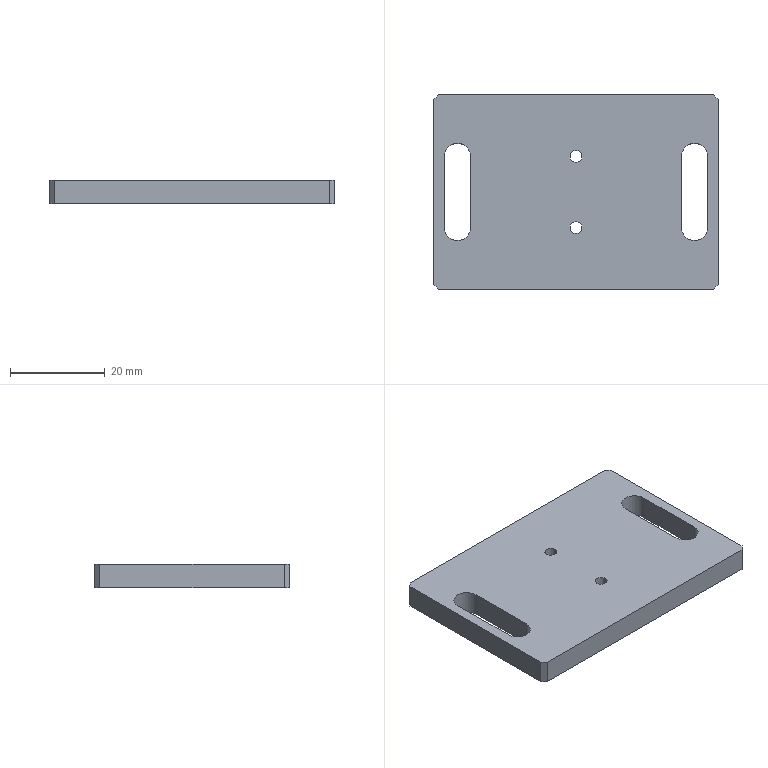Part | STEP file | KF-2212-010-050 | 1 solid | 22 faces | box 60 x 41 x 5 mm | volume 11178 mm3 | plane 14 | cylinder 8 | commonest cylinder face diameters 2.5 x4 5.5 x4
STEP:
#1=CARTESIAN_POINT('',(-1.25,7.5,0.));
#2=VERTEX_POINT('',#1);
#3=CARTESIAN_POINT('',(1.25,7.5,0.));
#4=VERTEX_POINT('',#3);
#5=CARTESIAN_POINT('',(0.,7.5,0.));
#6=DIRECTION('',(0.,0.,1.));
#7=DIRECTION('',(1.,0.,0.));
#8=AXIS2_PLACEMENT_3D('',#5,#6,#7);
#9=CIRCLE('',#8,1.25);
#10=EDGE_CURVE('',#2,#4,#9,.T.);
#11=ORIENTED_EDGE('',*,*,#10,.F.);
#12=CARTESIAN_POINT('',(-1.25,7.5,5.));
#13=VERTEX_POINT('',#12);
#14=CARTESIAN_POINT('',(-1.25,7.5,5.));
#15=DIRECTION('',(0.,0.,1.));
#16=VECTOR('',#15,1000.);
#17=LINE('',#14,#16);
#18=EDGE_CURVE('',#2,#13,#17,.T.);
#19=ORIENTED_EDGE('',*,*,#18,.T.);
#20=CARTESIAN_POINT('',(1.25,7.5,5.));
#21=VERTEX_POINT('',#20);
#22=CARTESIAN_POINT('',(0.,7.5,5.));
#23=DIRECTION('',(0.,0.,1.));
#24=DIRECTION('',(1.,0.,0.));
#25=AXIS2_PLACEMENT_3D('',#22,#23,#24);
#26=CIRCLE('',#25,1.25);
#27=EDGE_CURVE('',#13,#21,#26,.T.);
#28=ORIENTED_EDGE('',*,*,#27,.T.);
#29=CARTESIAN_POINT('',(1.25,7.5,5.));
#30=DIRECTION('',(0.,0.,1.));
#31=VECTOR('',#30,1000.);
#32=LINE('',#29,#31);
#33=EDGE_CURVE('',#4,#21,#32,.T.);
#34=ORIENTED_EDGE('',*,*,#33,.F.);
#35=EDGE_LOOP('',(#11,#19,#28,#34));
#36=FACE_OUTER_BOUND('',#35,.T.);
#37=CARTESIAN_POINT('',(0.,7.5,5.));
#38=DIRECTION('',(0.,0.,1.));
#39=DIRECTION('',(1.,0.,0.));
#40=AXIS2_PLACEMENT_3D('',#37,#38,#39);
#41=CYLINDRICAL_SURFACE('',#40,1.25);
#42=ADVANCED_FACE('',(#36),#41,.F.);
#43=CARTESIAN_POINT('',(-1.25,-7.5,0.));
#44=VERTEX_POINT('',#43);
#45=CARTESIAN_POINT('',(1.25,-7.5,0.));
#46=VERTEX_POINT('',#45);
#47=CARTESIAN_POINT('',(0.,-7.5,0.));
#48=DIRECTION('',(0.,0.,1.));
#49=DIRECTION('',(1.,0.,0.));
#50=AXIS2_PLACEMENT_3D('',#47,#48,#49);
#51=CIRCLE('',#50,1.25);
#52=EDGE_CURVE('',#44,#46,#51,.T.);
#53=ORIENTED_EDGE('',*,*,#52,.F.);
#54=CARTESIAN_POINT('',(-1.25,-7.5,5.));
#55=VERTEX_POINT('',#54);
#56=CARTESIAN_POINT('',(-1.25,-7.5,5.));
#57=DIRECTION('',(0.,0.,1.));
#58=VECTOR('',#57,1000.);
#59=LINE('',#56,#58);
#60=EDGE_CURVE('',#44,#55,#59,.T.);
#61=ORIENTED_EDGE('',*,*,#60,.T.);
#62=CARTESIAN_POINT('',(1.25,-7.5,5.));
#63=VERTEX_POINT('',#62);
#64=CARTESIAN_POINT('',(0.,-7.5,5.));
#65=DIRECTION('',(0.,0.,1.));
#66=DIRECTION('',(1.,0.,0.));
#67=AXIS2_PLACEMENT_3D('',#64,#65,#66);
#68=CIRCLE('',#67,1.25);
#69=EDGE_CURVE('',#55,#63,#68,.T.);
#70=ORIENTED_EDGE('',*,*,#69,.T.);
#71=CARTESIAN_POINT('',(1.25,-7.5,5.));
#72=DIRECTION('',(0.,0.,1.));
#73=VECTOR('',#72,1000.);
#74=LINE('',#71,#73);
#75=EDGE_CURVE('',#46,#63,#74,.T.);
#76=ORIENTED_EDGE('',*,*,#75,.F.);
#77=EDGE_LOOP('',(#53,#61,#70,#76));
#78=FACE_OUTER_BOUND('',#77,.T.);
#79=CARTESIAN_POINT('',(0.,-7.5,5.));
#80=DIRECTION('',(0.,0.,1.));
#81=DIRECTION('',(1.,0.,0.));
#82=AXIS2_PLACEMENT_3D('',#79,#80,#81);
#83=CYLINDRICAL_SURFACE('',#82,1.25);
#84=ADVANCED_FACE('',(#78),#83,.F.);
#85=CARTESIAN_POINT('',(-30.,19.5,5.));
#86=VERTEX_POINT('',#85);
#87=CARTESIAN_POINT('',(-30.,-19.5,5.));
#88=VERTEX_POINT('',#87);
#89=CARTESIAN_POINT('',(-30.,-20.5,5.));
#90=DIRECTION('',(0.,-1.,0.));
#91=VECTOR('',#90,1000.);
#92=LINE('',#89,#91);
#93=EDGE_CURVE('',#86,#88,#92,.T.);
#94=ORIENTED_EDGE('',*,*,#93,.F.);
#95=CARTESIAN_POINT('',(-30.,19.5,0.));
#96=VERTEX_POINT('',#95);
#97=CARTESIAN_POINT('',(-30.,19.5,5.));
#98=DIRECTION('',(0.,0.,-1.));
#99=VECTOR('',#98,1000.);
#100=LINE('',#97,#99);
#101=EDGE_CURVE('',#86,#96,#100,.T.);
#102=ORIENTED_EDGE('',*,*,#101,.T.);
#103=CARTESIAN_POINT('',(-30.,-19.5,0.));
#104=VERTEX_POINT('',#103);
#105=CARTESIAN_POINT('',(-30.,-20.5,0.));
#106=DIRECTION('',(0.,-1.,0.));
#107=VECTOR('',#106,1000.);
#108=LINE('',#105,#107);
#109=EDGE_CURVE('',#96,#104,#108,.T.);
#110=ORIENTED_EDGE('',*,*,#109,.T.);
#111=CARTESIAN_POINT('',(-30.,-19.5,5.));
#112=DIRECTION('',(0.,0.,1.));
#113=VECTOR('',#112,1000.);
#114=LINE('',#111,#113);
#115=EDGE_CURVE('',#104,#88,#114,.T.);
#116=ORIENTED_EDGE('',*,*,#115,.T.);
#117=EDGE_LOOP('',(#94,#102,#110,#116));
#118=FACE_OUTER_BOUND('',#117,.T.);
#119=CARTESIAN_POINT('',(-30.,-20.5,5.));
#120=DIRECTION('',(1.,0.,0.));
#121=DIRECTION('',(0.,0.,-1.));
#122=AXIS2_PLACEMENT_3D('',#119,#120,#121);
#123=PLANE('',#122);
#124=ADVANCED_FACE('',(#118),#123,.F.);
#125=CARTESIAN_POINT('',(-29.,-20.5,0.));
#126=VERTEX_POINT('',#125);
#127=CARTESIAN_POINT('',(29.,-20.5,0.));
#128=VERTEX_POINT('',#127);
#129=CARTESIAN_POINT('',(30.,-20.5,0.));
#130=DIRECTION('',(1.,0.,0.));
#131=VECTOR('',#130,1000.);
#132=LINE('',#129,#131);
#133=EDGE_CURVE('',#126,#128,#132,.T.);
#134=ORIENTED_EDGE('',*,*,#133,.T.);
#135=CARTESIAN_POINT('',(29.,-20.5,5.));
#136=VERTEX_POINT('',#135);
#137=CARTESIAN_POINT('',(29.,-20.5,5.));
#138=DIRECTION('',(0.,0.,1.));
#139=VECTOR('',#138,1000.);
#140=LINE('',#137,#139);
#141=EDGE_CURVE('',#128,#136,#140,.T.);
#142=ORIENTED_EDGE('',*,*,#141,.T.);
#143=CARTESIAN_POINT('',(-29.,-20.5,5.));
#144=VERTEX_POINT('',#143);
#145=CARTESIAN_POINT('',(30.,-20.5,5.));
#146=DIRECTION('',(1.,0.,0.));
#147=VECTOR('',#146,1000.);
#148=LINE('',#145,#147);
#149=EDGE_CURVE('',#144,#136,#148,.T.);
#150=ORIENTED_EDGE('',*,*,#149,.F.);
#151=CARTESIAN_POINT('',(-29.,-20.5,5.));
#152=DIRECTION('',(0.,0.,-1.));
#153=VECTOR('',#152,1000.);
#154=LINE('',#151,#153);
#155=EDGE_CURVE('',#144,#126,#154,.T.);
#156=ORIENTED_EDGE('',*,*,#155,.T.);
#157=EDGE_LOOP('',(#134,#142,#150,#156));
#158=FACE_OUTER_BOUND('',#157,.T.);
#159=CARTESIAN_POINT('',(30.,-20.5,5.));
#160=DIRECTION('',(0.,1.,0.));
#161=DIRECTION('',(-1.,0.,0.));
#162=AXIS2_PLACEMENT_3D('',#159,#160,#161);
#163=PLANE('',#162);
#164=ADVANCED_FACE('',(#158),#163,.F.);
#165=CARTESIAN_POINT('',(30.,-19.5,0.));
#166=VERTEX_POINT('',#165);
#167=CARTESIAN_POINT('',(30.,19.5,0.));
#168=VERTEX_POINT('',#167);
#169=CARTESIAN_POINT('',(30.,-20.5,0.));
#170=DIRECTION('',(0.,1.,0.));
#171=VECTOR('',#170,1000.);
#172=LINE('',#169,#171);
#173=EDGE_CURVE('',#166,#168,#172,.T.);
#174=ORIENTED_EDGE('',*,*,#173,.T.);
#175=CARTESIAN_POINT('',(30.,19.5,5.));
#176=VERTEX_POINT('',#175);
#177=CARTESIAN_POINT('',(30.,19.5,5.));
#178=DIRECTION('',(0.,0.,1.));
#179=VECTOR('',#178,1000.);
#180=LINE('',#177,#179);
#181=EDGE_CURVE('',#168,#176,#180,.T.);
#182=ORIENTED_EDGE('',*,*,#181,.T.);
#183=CARTESIAN_POINT('',(30.,-19.5,5.));
#184=VERTEX_POINT('',#183);
#185=CARTESIAN_POINT('',(30.,-20.5,5.));
#186=DIRECTION('',(0.,1.,0.));
#187=VECTOR('',#186,1000.);
#188=LINE('',#185,#187);
#189=EDGE_CURVE('',#184,#176,#188,.T.);
#190=ORIENTED_EDGE('',*,*,#189,.F.);
#191=CARTESIAN_POINT('',(30.,-19.5,5.));
#192=DIRECTION('',(0.,0.,-1.));
#193=VECTOR('',#192,1000.);
#194=LINE('',#191,#193);
#195=EDGE_CURVE('',#184,#166,#194,.T.);
#196=ORIENTED_EDGE('',*,*,#195,.T.);
#197=EDGE_LOOP('',(#174,#182,#190,#196));
#198=FACE_OUTER_BOUND('',#197,.T.);
#199=CARTESIAN_POINT('',(30.,-20.5,5.));
#200=DIRECTION('',(-1.,0.,0.));
#201=DIRECTION('',(0.,0.,1.));
#202=AXIS2_PLACEMENT_3D('',#199,#200,#201);
#203=PLANE('',#202);
#204=ADVANCED_FACE('',(#198),#203,.F.);
#205=CARTESIAN_POINT('',(29.,20.5,5.));
#206=VERTEX_POINT('',#205);
#207=CARTESIAN_POINT('',(-29.,20.5,5.));
#208=VERTEX_POINT('',#207);
#209=CARTESIAN_POINT('',(30.,20.5,5.));
#210=DIRECTION('',(-1.,0.,0.));
#211=VECTOR('',#210,1000.);
#212=LINE('',#209,#211);
#213=EDGE_CURVE('',#206,#208,#212,.T.);
#214=ORIENTED_EDGE('',*,*,#213,.F.);
#215=CARTESIAN_POINT('',(29.,20.5,0.));
#216=VERTEX_POINT('',#215);
#217=CARTESIAN_POINT('',(29.,20.5,5.));
#218=DIRECTION('',(0.,0.,-1.));
#219=VECTOR('',#218,1000.);
#220=LINE('',#217,#219);
#221=EDGE_CURVE('',#206,#216,#220,.T.);
#222=ORIENTED_EDGE('',*,*,#221,.T.);
#223=CARTESIAN_POINT('',(-29.,20.5,0.));
#224=VERTEX_POINT('',#223);
#225=CARTESIAN_POINT('',(30.,20.5,0.));
#226=DIRECTION('',(-1.,0.,0.));
#227=VECTOR('',#226,1000.);
#228=LINE('',#225,#227);
#229=EDGE_CURVE('',#216,#224,#228,.T.);
#230=ORIENTED_EDGE('',*,*,#229,.T.);
#231=CARTESIAN_POINT('',(-29.,20.5,5.));
#232=DIRECTION('',(0.,0.,1.));
#233=VECTOR('',#232,1000.);
#234=LINE('',#231,#233);
#235=EDGE_CURVE('',#224,#208,#234,.T.);
#236=ORIENTED_EDGE('',*,*,#235,.T.);
#237=EDGE_LOOP('',(#214,#222,#230,#236));
#238=FACE_OUTER_BOUND('',#237,.T.);
#239=CARTESIAN_POINT('',(30.,20.5,5.));
#240=DIRECTION('',(0.,-1.,0.));
#241=DIRECTION('',(1.,0.,0.));
#242=AXIS2_PLACEMENT_3D('',#239,#240,#241);
#243=PLANE('',#242);
#244=ADVANCED_FACE('',(#238),#243,.F.);
#245=CARTESIAN_POINT('',(-27.75,-7.5,5.));
#246=VERTEX_POINT('',#245);
#247=CARTESIAN_POINT('',(-22.25,-7.5,5.));
#248=VERTEX_POINT('',#247);
#249=CARTESIAN_POINT('',(-25.,-7.5,5.));
#250=DIRECTION('',(0.,0.,1.));
#251=DIRECTION('',(1.,0.,0.));
#252=AXIS2_PLACEMENT_3D('',#249,#250,#251);
#253=CIRCLE('',#252,2.75);
#254=EDGE_CURVE('',#246,#248,#253,.T.);
#255=ORIENTED_EDGE('',*,*,#254,.F.);
#256=CARTESIAN_POINT('',(-27.75,7.5,5.));
#257=VERTEX_POINT('',#256);
#258=CARTESIAN_POINT('',(-27.75,-7.5,5.));
#259=DIRECTION('',(0.,-1.,0.));
#260=VECTOR('',#259,1000.);
#261=LINE('',#258,#260);
#262=EDGE_CURVE('',#257,#246,#261,.T.);
#263=ORIENTED_EDGE('',*,*,#262,.F.);
#264=CARTESIAN_POINT('',(-22.25,7.5,5.));
#265=VERTEX_POINT('',#264);
#266=CARTESIAN_POINT('',(-25.,7.5,5.));
#267=DIRECTION('',(0.,0.,1.));
#268=DIRECTION('',(1.,0.,0.));
#269=AXIS2_PLACEMENT_3D('',#266,#267,#268);
#270=CIRCLE('',#269,2.75);
#271=EDGE_CURVE('',#265,#257,#270,.T.);
#272=ORIENTED_EDGE('',*,*,#271,.F.);
#273=CARTESIAN_POINT('',(-22.25,-7.5,5.));
#274=DIRECTION('',(0.,1.,0.));
#275=VECTOR('',#274,1000.);
#276=LINE('',#273,#275);
#277=EDGE_CURVE('',#248,#265,#276,.T.);
#278=ORIENTED_EDGE('',*,*,#277,.F.);
#279=EDGE_LOOP('',(#255,#263,#272,#278));
#280=FACE_BOUND('',#279,.T.);
#281=CARTESIAN_POINT('',(27.75,7.5,5.));
#282=VERTEX_POINT('',#281);
#283=CARTESIAN_POINT('',(22.25,7.5,5.));
#284=VERTEX_POINT('',#283);
#285=CARTESIAN_POINT('',(25.,7.5,5.));
#286=DIRECTION('',(0.,0.,1.));
#287=DIRECTION('',(1.,0.,0.));
#288=AXIS2_PLACEMENT_3D('',#285,#286,#287);
#289=CIRCLE('',#288,2.75);
#290=EDGE_CURVE('',#282,#284,#289,.T.);
#291=ORIENTED_EDGE('',*,*,#290,.F.);
#292=CARTESIAN_POINT('',(27.75,-7.5,5.));
#293=VERTEX_POINT('',#292);
#294=CARTESIAN_POINT('',(27.75,7.5,5.));
#295=DIRECTION('',(0.,1.,0.));
#296=VECTOR('',#295,1000.);
#297=LINE('',#294,#296);
#298=EDGE_CURVE('',#293,#282,#297,.T.);
#299=ORIENTED_EDGE('',*,*,#298,.F.);
#300=CARTESIAN_POINT('',(22.25,-7.5,5.));
#301=VERTEX_POINT('',#300);
#302=CARTESIAN_POINT('',(25.,-7.5,5.));
#303=DIRECTION('',(0.,0.,1.));
#304=DIRECTION('',(1.,0.,0.));
#305=AXIS2_PLACEMENT_3D('',#302,#303,#304);
#306=CIRCLE('',#305,2.75);
#307=EDGE_CURVE('',#301,#293,#306,.T.);
#308=ORIENTED_EDGE('',*,*,#307,.F.);
#309=CARTESIAN_POINT('',(22.25,7.5,5.));
#310=DIRECTION('',(0.,-1.,0.));
#311=VECTOR('',#310,1000.);
#312=LINE('',#309,#311);
#313=EDGE_CURVE('',#284,#301,#312,.T.);
#314=ORIENTED_EDGE('',*,*,#313,.F.);
#315=EDGE_LOOP('',(#291,#299,#308,#314));
#316=FACE_BOUND('',#315,.T.);
#317=CARTESIAN_POINT('',(0.,7.5,5.));
#318=DIRECTION('',(0.,0.,1.));
#319=DIRECTION('',(1.,0.,0.));
#320=AXIS2_PLACEMENT_3D('',#317,#318,#319);
#321=CIRCLE('',#320,1.25);
#322=EDGE_CURVE('',#21,#13,#321,.T.);
#323=ORIENTED_EDGE('',*,*,#322,.F.);
#324=ORIENTED_EDGE('',*,*,#27,.F.);
#325=EDGE_LOOP('',(#323,#324));
#326=FACE_BOUND('',#325,.T.);
#327=CARTESIAN_POINT('',(0.,-7.5,5.));
#328=DIRECTION('',(0.,0.,1.));
#329=DIRECTION('',(1.,0.,0.));
#330=AXIS2_PLACEMENT_3D('',#327,#328,#329);
#331=CIRCLE('',#330,1.25);
#332=EDGE_CURVE('',#63,#55,#331,.T.);
#333=ORIENTED_EDGE('',*,*,#332,.F.);
#334=ORIENTED_EDGE('',*,*,#69,.F.);
#335=EDGE_LOOP('',(#333,#334));
#336=FACE_BOUND('',#335,.T.);
#337=ORIENTED_EDGE('',*,*,#189,.T.);
#338=CARTESIAN_POINT('',(24.75,24.75,5.));
#339=DIRECTION('',(-0.7071,0.7071,0.));
#340=VECTOR('',#339,1000.);
#341=LINE('',#338,#340);
#342=EDGE_CURVE('',#176,#206,#341,.T.);
#343=ORIENTED_EDGE('',*,*,#342,.T.);
#344=ORIENTED_EDGE('',*,*,#213,.T.);
#345=CARTESIAN_POINT('',(-24.75,24.75,5.));
#346=DIRECTION('',(-0.7071,-0.7071,0.));
#347=VECTOR('',#346,1000.);
#348=LINE('',#345,#347);
#349=EDGE_CURVE('',#208,#86,#348,.T.);
#350=ORIENTED_EDGE('',*,*,#349,.T.);
#351=ORIENTED_EDGE('',*,*,#93,.T.);
#352=CARTESIAN_POINT('',(-24.75,-24.75,5.));
#353=DIRECTION('',(0.7071,-0.7071,0.));
#354=VECTOR('',#353,1000.);
#355=LINE('',#352,#354);
#356=EDGE_CURVE('',#88,#144,#355,.T.);
#357=ORIENTED_EDGE('',*,*,#356,.T.);
#358=ORIENTED_EDGE('',*,*,#149,.T.);
#359=CARTESIAN_POINT('',(24.75,-24.75,5.));
#360=DIRECTION('',(0.7071,0.7071,0.));
#361=VECTOR('',#360,1000.);
#362=LINE('',#359,#361);
#363=EDGE_CURVE('',#136,#184,#362,.T.);
#364=ORIENTED_EDGE('',*,*,#363,.T.);
#365=EDGE_LOOP('',(#337,#343,#344,#350,#351,#357,#358,#364));
#366=FACE_OUTER_BOUND('',#365,.T.);
#367=CARTESIAN_POINT('',(0.,0.,5.));
#368=DIRECTION('',(0.,0.,1.));
#369=DIRECTION('',(1.,0.,0.));
#370=AXIS2_PLACEMENT_3D('',#367,#368,#369);
#371=PLANE('',#370);
#372=ADVANCED_FACE('',(#280,#316,#326,#336,#366),#371,.T.);
#373=CARTESIAN_POINT('',(-27.75,7.5,0.));
#374=VERTEX_POINT('',#373);
#375=CARTESIAN_POINT('',(-27.75,-7.5,0.));
#376=VERTEX_POINT('',#375);
#377=CARTESIAN_POINT('',(-27.75,-7.5,0.));
#378=DIRECTION('',(0.,-1.,0.));
#379=VECTOR('',#378,1000.);
#380=LINE('',#377,#379);
#381=EDGE_CURVE('',#374,#376,#380,.T.);
#382=ORIENTED_EDGE('',*,*,#381,.T.);
#383=CARTESIAN_POINT('',(-22.25,-7.5,0.));
#384=VERTEX_POINT('',#383);
#385=CARTESIAN_POINT('',(-25.,-7.5,0.));
#386=DIRECTION('',(0.,0.,1.));
#387=DIRECTION('',(1.,0.,0.));
#388=AXIS2_PLACEMENT_3D('',#385,#386,#387);
#389=CIRCLE('',#388,2.75);
#390=EDGE_CURVE('',#376,#384,#389,.T.);
#391=ORIENTED_EDGE('',*,*,#390,.T.);
#392=CARTESIAN_POINT('',(-22.25,7.5,0.));
#393=VERTEX_POINT('',#392);
#394=CARTESIAN_POINT('',(-22.25,-7.5,0.));
#395=DIRECTION('',(0.,1.,0.));
#396=VECTOR('',#395,1000.);
#397=LINE('',#394,#396);
#398=EDGE_CURVE('',#384,#393,#397,.T.);
#399=ORIENTED_EDGE('',*,*,#398,.T.);
#400=CARTESIAN_POINT('',(-25.,7.5,0.));
#401=DIRECTION('',(0.,0.,1.));
#402=DIRECTION('',(1.,0.,0.));
#403=AXIS2_PLACEMENT_3D('',#400,#401,#402);
#404=CIRCLE('',#403,2.75);
#405=EDGE_CURVE('',#393,#374,#404,.T.);
#406=ORIENTED_EDGE('',*,*,#405,.T.);
#407=EDGE_LOOP('',(#382,#391,#399,#406));
#408=FACE_BOUND('',#407,.T.);
#409=CARTESIAN_POINT('',(27.75,-7.5,0.));
#410=VERTEX_POINT('',#409);
#411=CARTESIAN_POINT('',(27.75,7.5,0.));
#412=VERTEX_POINT('',#411);
#413=CARTESIAN_POINT('',(27.75,7.5,0.));
#414=DIRECTION('',(0.,1.,0.));
#415=VECTOR('',#414,1000.);
#416=LINE('',#413,#415);
#417=EDGE_CURVE('',#410,#412,#416,.T.);
#418=ORIENTED_EDGE('',*,*,#417,.T.);
#419=CARTESIAN_POINT('',(22.25,7.5,0.));
#420=VERTEX_POINT('',#419);
#421=CARTESIAN_POINT('',(25.,7.5,0.));
#422=DIRECTION('',(0.,0.,1.));
#423=DIRECTION('',(1.,0.,0.));
#424=AXIS2_PLACEMENT_3D('',#421,#422,#423);
#425=CIRCLE('',#424,2.75);
#426=EDGE_CURVE('',#412,#420,#425,.T.);
#427=ORIENTED_EDGE('',*,*,#426,.T.);
#428=CARTESIAN_POINT('',(22.25,-7.5,0.));
#429=VERTEX_POINT('',#428);
#430=CARTESIAN_POINT('',(22.25,7.5,0.));
#431=DIRECTION('',(0.,-1.,0.));
#432=VECTOR('',#431,1000.);
#433=LINE('',#430,#432);
#434=EDGE_CURVE('',#420,#429,#433,.T.);
#435=ORIENTED_EDGE('',*,*,#434,.T.);
#436=CARTESIAN_POINT('',(25.,-7.5,0.));
#437=DIRECTION('',(0.,0.,1.));
#438=DIRECTION('',(1.,0.,0.));
#439=AXIS2_PLACEMENT_3D('',#436,#437,#438);
#440=CIRCLE('',#439,2.75);
#441=EDGE_CURVE('',#429,#410,#440,.T.);
#442=ORIENTED_EDGE('',*,*,#441,.T.);
#443=EDGE_LOOP('',(#418,#427,#435,#442));
#444=FACE_BOUND('',#443,.T.);
#445=CARTESIAN_POINT('',(0.,7.5,0.));
#446=DIRECTION('',(0.,0.,1.));
#447=DIRECTION('',(1.,0.,0.));
#448=AXIS2_PLACEMENT_3D('',#445,#446,#447);
#449=CIRCLE('',#448,1.25);
#450=EDGE_CURVE('',#4,#2,#449,.T.);
#451=ORIENTED_EDGE('',*,*,#450,.T.);
#452=ORIENTED_EDGE('',*,*,#10,.T.);
#453=EDGE_LOOP('',(#451,#452));
#454=FACE_BOUND('',#453,.T.);
#455=CARTESIAN_POINT('',(0.,-7.5,0.));
#456=DIRECTION('',(0.,0.,1.));
#457=DIRECTION('',(1.,0.,0.));
#458=AXIS2_PLACEMENT_3D('',#455,#456,#457);
#459=CIRCLE('',#458,1.25);
#460=EDGE_CURVE('',#46,#44,#459,.T.);
#461=ORIENTED_EDGE('',*,*,#460,.T.);
#462=ORIENTED_EDGE('',*,*,#52,.T.);
#463=EDGE_LOOP('',(#461,#462));
#464=FACE_BOUND('',#463,.T.);
#465=ORIENTED_EDGE('',*,*,#229,.F.);
#466=CARTESIAN_POINT('',(29.,20.5,0.));
#467=DIRECTION('',(0.7071,-0.7071,0.));
#468=VECTOR('',#467,1000.);
#469=LINE('',#466,#468);
#470=EDGE_CURVE('',#216,#168,#469,.T.);
#471=ORIENTED_EDGE('',*,*,#470,.T.);
#472=ORIENTED_EDGE('',*,*,#173,.F.);
#473=CARTESIAN_POINT('',(30.,-19.5,0.));
#474=DIRECTION('',(-0.7071,-0.7071,0.));
#475=VECTOR('',#474,1000.);
#476=LINE('',#473,#475);
#477=EDGE_CURVE('',#166,#128,#476,.T.);
#478=ORIENTED_EDGE('',*,*,#477,.T.);
#479=ORIENTED_EDGE('',*,*,#133,.F.);
#480=CARTESIAN_POINT('',(-29.,-20.5,0.));
#481=DIRECTION('',(-0.7071,0.7071,0.));
#482=VECTOR('',#481,1000.);
#483=LINE('',#480,#482);
#484=EDGE_CURVE('',#126,#104,#483,.T.);
#485=ORIENTED_EDGE('',*,*,#484,.T.);
#486=ORIENTED_EDGE('',*,*,#109,.F.);
#487=CARTESIAN_POINT('',(-30.,19.5,0.));
#488=DIRECTION('',(0.7071,0.7071,0.));
#489=VECTOR('',#488,1000.);
#490=LINE('',#487,#489);
#491=EDGE_CURVE('',#96,#224,#490,.T.);
#492=ORIENTED_EDGE('',*,*,#491,.T.);
#493=EDGE_LOOP('',(#465,#471,#472,#478,#479,#485,#486,#492));
#494=FACE_OUTER_BOUND('',#493,.T.);
#495=CARTESIAN_POINT('',(0.,0.,0.));
#496=DIRECTION('',(0.,0.,1.));
#497=DIRECTION('',(1.,0.,0.));
#498=AXIS2_PLACEMENT_3D('',#495,#496,#497);
#499=PLANE('',#498);
#500=ADVANCED_FACE('',(#408,#444,#454,#464,#494),#499,.F.);
#501=ORIENTED_EDGE('',*,*,#60,.F.);
#502=ORIENTED_EDGE('',*,*,#460,.F.);
#503=ORIENTED_EDGE('',*,*,#75,.T.);
#504=ORIENTED_EDGE('',*,*,#332,.T.);
#505=EDGE_LOOP('',(#501,#502,#503,#504));
#506=FACE_OUTER_BOUND('',#505,.T.);
#507=CARTESIAN_POINT('',(0.,-7.5,5.));
#508=DIRECTION('',(0.,0.,1.));
#509=DIRECTION('',(1.,0.,0.));
#510=AXIS2_PLACEMENT_3D('',#507,#508,#509);
#511=CYLINDRICAL_SURFACE('',#510,1.25);
#512=ADVANCED_FACE('',(#506),#511,.F.);
#513=ORIENTED_EDGE('',*,*,#18,.F.);
#514=ORIENTED_EDGE('',*,*,#450,.F.);
#515=ORIENTED_EDGE('',*,*,#33,.T.);
#516=ORIENTED_EDGE('',*,*,#322,.T.);
#517=EDGE_LOOP('',(#513,#514,#515,#516));
#518=FACE_OUTER_BOUND('',#517,.T.);
#519=CARTESIAN_POINT('',(0.,7.5,5.));
#520=DIRECTION('',(0.,0.,1.));
#521=DIRECTION('',(1.,0.,0.));
#522=AXIS2_PLACEMENT_3D('',#519,#520,#521);
#523=CYLINDRICAL_SURFACE('',#522,1.25);
#524=ADVANCED_FACE('',(#518),#523,.F.);
#525=ORIENTED_EDGE('',*,*,#342,.F.);
#526=ORIENTED_EDGE('',*,*,#181,.F.);
#527=ORIENTED_EDGE('',*,*,#470,.F.);
#528=ORIENTED_EDGE('',*,*,#221,.F.);
#529=EDGE_LOOP('',(#525,#526,#527,#528));
#530=FACE_OUTER_BOUND('',#529,.T.);
#531=CARTESIAN_POINT('',(29.,20.5,5.));
#532=DIRECTION('',(-0.7071,-0.7071,0.));
#533=DIRECTION('',(0.,0.,-1.));
#534=AXIS2_PLACEMENT_3D('',#531,#532,#533);
#535=PLANE('',#534);
#536=ADVANCED_FACE('',(#530),#535,.F.);
#537=ORIENTED_EDGE('',*,*,#363,.F.);
#538=ORIENTED_EDGE('',*,*,#141,.F.);
#539=ORIENTED_EDGE('',*,*,#477,.F.);
#540=ORIENTED_EDGE('',*,*,#195,.F.);
#541=EDGE_LOOP('',(#537,#538,#539,#540));
#542=FACE_OUTER_BOUND('',#541,.T.);
#543=CARTESIAN_POINT('',(30.,-19.5,5.));
#544=DIRECTION('',(-0.7071,0.7071,0.));
#545=DIRECTION('',(0.,0.,-1.));
#546=AXIS2_PLACEMENT_3D('',#543,#544,#545);
#547=PLANE('',#546);
#548=ADVANCED_FACE('',(#542),#547,.F.);
#549=ORIENTED_EDGE('',*,*,#349,.F.);
#550=ORIENTED_EDGE('',*,*,#235,.F.);
#551=ORIENTED_EDGE('',*,*,#491,.F.);
#552=ORIENTED_EDGE('',*,*,#101,.F.);
#553=EDGE_LOOP('',(#549,#550,#551,#552));
#554=FACE_OUTER_BOUND('',#553,.T.);
#555=CARTESIAN_POINT('',(-30.,19.5,5.));
#556=DIRECTION('',(0.7071,-0.7071,0.));
#557=DIRECTION('',(0.,0.,-1.));
#558=AXIS2_PLACEMENT_3D('',#555,#556,#557);
#559=PLANE('',#558);
#560=ADVANCED_FACE('',(#554),#559,.F.);
#561=ORIENTED_EDGE('',*,*,#356,.F.);
#562=ORIENTED_EDGE('',*,*,#115,.F.);
#563=ORIENTED_EDGE('',*,*,#484,.F.);
#564=ORIENTED_EDGE('',*,*,#155,.F.);
#565=EDGE_LOOP('',(#561,#562,#563,#564));
#566=FACE_OUTER_BOUND('',#565,.T.);
#567=CARTESIAN_POINT('',(-29.,-20.5,5.));
#568=DIRECTION('',(0.7071,0.7071,0.));
#569=DIRECTION('',(0.,0.,-1.));
#570=AXIS2_PLACEMENT_3D('',#567,#568,#569);
#571=PLANE('',#570);
#572=ADVANCED_FACE('',(#566),#571,.F.);
#573=ORIENTED_EDGE('',*,*,#290,.T.);
#574=CARTESIAN_POINT('',(22.25,7.5,0.));
#575=DIRECTION('',(0.,0.,1.));
#576=VECTOR('',#575,1000.);
#577=LINE('',#574,#576);
#578=EDGE_CURVE('',#420,#284,#577,.T.);
#579=ORIENTED_EDGE('',*,*,#578,.F.);
#580=ORIENTED_EDGE('',*,*,#426,.F.);
#581=CARTESIAN_POINT('',(27.75,7.5,0.));
#582=DIRECTION('',(0.,0.,1.));
#583=VECTOR('',#582,1000.);
#584=LINE('',#581,#583);
#585=EDGE_CURVE('',#412,#282,#584,.T.);
#586=ORIENTED_EDGE('',*,*,#585,.T.);
#587=EDGE_LOOP('',(#573,#579,#580,#586));
#588=FACE_OUTER_BOUND('',#587,.T.);
#589=CARTESIAN_POINT('',(25.,7.5,0.));
#590=DIRECTION('',(0.,0.,1.));
#591=DIRECTION('',(1.,0.,0.));
#592=AXIS2_PLACEMENT_3D('',#589,#590,#591);
#593=CYLINDRICAL_SURFACE('',#592,2.75);
#594=ADVANCED_FACE('',(#588),#593,.F.);
#595=ORIENTED_EDGE('',*,*,#298,.T.);
#596=ORIENTED_EDGE('',*,*,#585,.F.);
#597=ORIENTED_EDGE('',*,*,#417,.F.);
#598=CARTESIAN_POINT('',(27.75,-7.5,0.));
#599=DIRECTION('',(0.,0.,1.));
#600=VECTOR('',#599,1000.);
#601=LINE('',#598,#600);
#602=EDGE_CURVE('',#410,#293,#601,.T.);
#603=ORIENTED_EDGE('',*,*,#602,.T.);
#604=EDGE_LOOP('',(#595,#596,#597,#603));
#605=FACE_OUTER_BOUND('',#604,.T.);
#606=CARTESIAN_POINT('',(27.75,7.5,0.));
#607=DIRECTION('',(1.,0.,0.));
#608=DIRECTION('',(0.,1.,0.));
#609=AXIS2_PLACEMENT_3D('',#606,#607,#608);
#610=PLANE('',#609);
#611=ADVANCED_FACE('',(#605),#610,.F.);
#612=ORIENTED_EDGE('',*,*,#307,.T.);
#613=ORIENTED_EDGE('',*,*,#602,.F.);
#614=ORIENTED_EDGE('',*,*,#441,.F.);
#615=CARTESIAN_POINT('',(22.25,-7.5,0.));
#616=DIRECTION('',(0.,0.,1.));
#617=VECTOR('',#616,1000.);
#618=LINE('',#615,#617);
#619=EDGE_CURVE('',#429,#301,#618,.T.);
#620=ORIENTED_EDGE('',*,*,#619,.T.);
#621=EDGE_LOOP('',(#612,#613,#614,#620));
#622=FACE_OUTER_BOUND('',#621,.T.);
#623=CARTESIAN_POINT('',(25.,-7.5,0.));
#624=DIRECTION('',(0.,0.,1.));
#625=DIRECTION('',(1.,0.,0.));
#626=AXIS2_PLACEMENT_3D('',#623,#624,#625);
#627=CYLINDRICAL_SURFACE('',#626,2.75);
#628=ADVANCED_FACE('',(#622),#627,.F.);
#629=ORIENTED_EDGE('',*,*,#313,.T.);
#630=ORIENTED_EDGE('',*,*,#619,.F.);
#631=ORIENTED_EDGE('',*,*,#434,.F.);
#632=ORIENTED_EDGE('',*,*,#578,.T.);
#633=EDGE_LOOP('',(#629,#630,#631,#632));
#634=FACE_OUTER_BOUND('',#633,.T.);
#635=CARTESIAN_POINT('',(22.25,7.5,0.));
#636=DIRECTION('',(-1.,0.,0.));
#637=DIRECTION('',(0.,-1.,0.));
#638=AXIS2_PLACEMENT_3D('',#635,#636,#637);
#639=PLANE('',#638);
#640=ADVANCED_FACE('',(#634),#639,.F.);
#641=ORIENTED_EDGE('',*,*,#254,.T.);
#642=CARTESIAN_POINT('',(-22.25,-7.5,0.));
#643=DIRECTION('',(0.,0.,1.));
#644=VECTOR('',#643,1000.);
#645=LINE('',#642,#644);
#646=EDGE_CURVE('',#384,#248,#645,.T.);
#647=ORIENTED_EDGE('',*,*,#646,.F.);
#648=ORIENTED_EDGE('',*,*,#390,.F.);
#649=CARTESIAN_POINT('',(-27.75,-7.5,0.));
#650=DIRECTION('',(0.,0.,1.));
#651=VECTOR('',#650,1000.);
#652=LINE('',#649,#651);
#653=EDGE_CURVE('',#376,#246,#652,.T.);
#654=ORIENTED_EDGE('',*,*,#653,.T.);
#655=EDGE_LOOP('',(#641,#647,#648,#654));
#656=FACE_OUTER_BOUND('',#655,.T.);
#657=CARTESIAN_POINT('',(-25.,-7.5,0.));
#658=DIRECTION('',(0.,0.,1.));
#659=DIRECTION('',(1.,0.,0.));
#660=AXIS2_PLACEMENT_3D('',#657,#658,#659);
#661=CYLINDRICAL_SURFACE('',#660,2.75);
#662=ADVANCED_FACE('',(#656),#661,.F.);
#663=ORIENTED_EDGE('',*,*,#262,.T.);
#664=ORIENTED_EDGE('',*,*,#653,.F.);
#665=ORIENTED_EDGE('',*,*,#381,.F.);
#666=CARTESIAN_POINT('',(-27.75,7.5,0.));
#667=DIRECTION('',(0.,0.,1.));
#668=VECTOR('',#667,1000.);
#669=LINE('',#666,#668);
#670=EDGE_CURVE('',#374,#257,#669,.T.);
#671=ORIENTED_EDGE('',*,*,#670,.T.);
#672=EDGE_LOOP('',(#663,#664,#665,#671));
#673=FACE_OUTER_BOUND('',#672,.T.);
#674=CARTESIAN_POINT('',(-27.75,-7.5,0.));
#675=DIRECTION('',(-1.,0.,0.));
#676=DIRECTION('',(0.,-1.,0.));
#677=AXIS2_PLACEMENT_3D('',#674,#675,#676);
#678=PLANE('',#677);
#679=ADVANCED_FACE('',(#673),#678,.F.);
#680=ORIENTED_EDGE('',*,*,#271,.T.);
#681=ORIENTED_EDGE('',*,*,#670,.F.);
#682=ORIENTED_EDGE('',*,*,#405,.F.);
#683=CARTESIAN_POINT('',(-22.25,7.5,0.));
#684=DIRECTION('',(0.,0.,1.));
#685=VECTOR('',#684,1000.);
#686=LINE('',#683,#685);
#687=EDGE_CURVE('',#393,#265,#686,.T.);
#688=ORIENTED_EDGE('',*,*,#687,.T.);
#689=EDGE_LOOP('',(#680,#681,#682,#688));
#690=FACE_OUTER_BOUND('',#689,.T.);
#691=CARTESIAN_POINT('',(-25.,7.5,0.));
#692=DIRECTION('',(0.,0.,1.));
#693=DIRECTION('',(1.,0.,0.));
#694=AXIS2_PLACEMENT_3D('',#691,#692,#693);
#695=CYLINDRICAL_SURFACE('',#694,2.75);
#696=ADVANCED_FACE('',(#690),#695,.F.);
#697=ORIENTED_EDGE('',*,*,#277,.T.);
#698=ORIENTED_EDGE('',*,*,#687,.F.);
#699=ORIENTED_EDGE('',*,*,#398,.F.);
#700=ORIENTED_EDGE('',*,*,#646,.T.);
#701=EDGE_LOOP('',(#697,#698,#699,#700));
#702=FACE_OUTER_BOUND('',#701,.T.);
#703=CARTESIAN_POINT('',(-22.25,-7.5,0.));
#704=DIRECTION('',(1.,0.,0.));
#705=DIRECTION('',(0.,1.,0.));
#706=AXIS2_PLACEMENT_3D('',#703,#704,#705);
#707=PLANE('',#706);
#708=ADVANCED_FACE('',(#702),#707,.F.);
#709=CLOSED_SHELL('',(#42,#84,#124,#164,#204,#244,#372,#500,#512,#524,#536,#548,#560,#572,#594,#611,#628,#640,#662,#679,#696,#708));
#710=MANIFOLD_SOLID_BREP('',#709);
#711=CARTESIAN_POINT('',(0.,0.,0.));
#712=DIRECTION('',(0.,0.,1.));
#713=DIRECTION('',(1.,0.,0.));
#714=AXIS2_PLACEMENT_3D('',#711,#712,#713);
#715=(LENGTH_UNIT()NAMED_UNIT(*)SI_UNIT(.MILLI.,.METRE.));
#716=UNCERTAINTY_MEASURE_WITH_UNIT(LENGTH_MEASURE(0.00001),#715,'','');
#717=(NAMED_UNIT(*)PLANE_ANGLE_UNIT()SI_UNIT($,.RADIAN.));
#718=(NAMED_UNIT(*)SI_UNIT($,.STERADIAN.)SOLID_ANGLE_UNIT());
#719=(GEOMETRIC_REPRESENTATION_CONTEXT(3)GLOBAL_UNCERTAINTY_ASSIGNED_CONTEXT((#716))GLOBAL_UNIT_ASSIGNED_CONTEXT((#715,#717,#718))REPRESENTATION_CONTEXT('',''));
#720=ADVANCED_BREP_SHAPE_REPRESENTATION('',(#710,#714),#719);